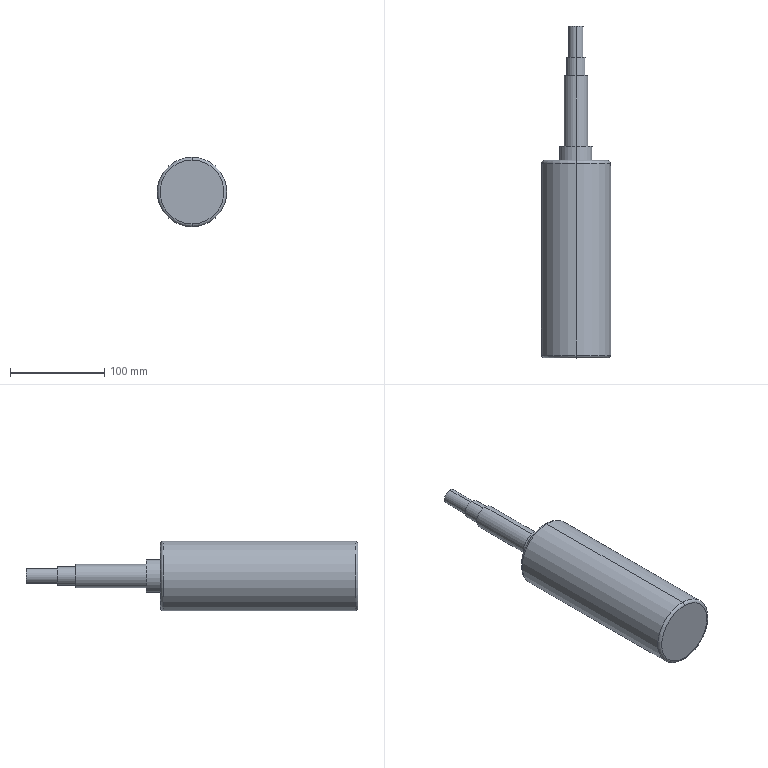Part | SolidWorks | features ICE 4, Extrusion 1, Fillet 1 | 1 solid | 20 faces | box 74 x 353 x 74 mm | volume 966460 mm3 | cylinder 10 | plane 6 | torus 4 | commonest cylinder face diameters 16 x2 20 x2 25 x2 35 x2 74 x2
STEP:
#1=CARTESIAN_POINT('',(0.,102.,-37.));
#2=VERTEX_POINT('',#1);
#3=CARTESIAN_POINT('',(0.,102.,37.));
#4=VERTEX_POINT('',#3);
#5=CARTESIAN_POINT('',(0.,102.,0.));
#6=DIRECTION('',(0.,-1.,0.));
#7=DIRECTION('',(0.,0.,1.));
#8=AXIS2_PLACEMENT_3D('',#5,#6,#7);
#9=CIRCLE('',#8,37.);
#10=EDGE_CURVE('',#2,#4,#9,.T.);
#11=ORIENTED_EDGE('',*,*,#10,.F.);
#12=CARTESIAN_POINT('',(0.,105.,-34.));
#13=VERTEX_POINT('',#12);
#14=CARTESIAN_POINT('',(0.,102.,-34.));
#15=DIRECTION('',(1.,0.,0.));
#16=DIRECTION('',(0.,0.,-1.));
#17=AXIS2_PLACEMENT_3D('',#14,#15,#16);
#18=CIRCLE('',#17,3.);
#19=EDGE_CURVE('',#2,#13,#18,.T.);
#20=ORIENTED_EDGE('',*,*,#19,.T.);
#21=CARTESIAN_POINT('',(0.,105.,34.));
#22=VERTEX_POINT('',#21);
#23=CARTESIAN_POINT('',(0.,105.,0.));
#24=DIRECTION('',(0.,1.,0.));
#25=DIRECTION('',(0.,0.,1.));
#26=AXIS2_PLACEMENT_3D('',#23,#24,#25);
#27=CIRCLE('',#26,34.);
#28=EDGE_CURVE('',#22,#13,#27,.T.);
#29=ORIENTED_EDGE('',*,*,#28,.F.);
#30=CARTESIAN_POINT('',(0.,102.,34.));
#31=DIRECTION('',(-1.,0.,0.));
#32=DIRECTION('',(0.,0.,1.));
#33=AXIS2_PLACEMENT_3D('',#30,#31,#32);
#34=CIRCLE('',#33,3.);
#35=EDGE_CURVE('',#4,#22,#34,.T.);
#36=ORIENTED_EDGE('',*,*,#35,.F.);
#37=EDGE_LOOP('',(#11,#20,#29,#36));
#38=FACE_OUTER_BOUND('',#37,.T.);
#39=CARTESIAN_POINT('',(0.,102.,0.));
#40=DIRECTION('',(0.,1.,0.));
#41=DIRECTION('',(0.,0.,1.));
#42=AXIS2_PLACEMENT_3D('',#39,#40,#41);
#43=TOROIDAL_SURFACE('',#42,34.,3.);
#44=ADVANCED_FACE('',(#38),#43,.T.);
#45=CARTESIAN_POINT('',(0.,-105.,-34.));
#46=VERTEX_POINT('',#45);
#47=CARTESIAN_POINT('',(0.,-105.,34.));
#48=VERTEX_POINT('',#47);
#49=CARTESIAN_POINT('',(0.,-105.,0.));
#50=DIRECTION('',(0.,-1.,0.));
#51=DIRECTION('',(0.,0.,1.));
#52=AXIS2_PLACEMENT_3D('',#49,#50,#51);
#53=CIRCLE('',#52,34.);
#54=EDGE_CURVE('',#46,#48,#53,.T.);
#55=ORIENTED_EDGE('',*,*,#54,.F.);
#56=CARTESIAN_POINT('',(0.,-102.,-37.));
#57=VERTEX_POINT('',#56);
#58=CARTESIAN_POINT('',(0.,-102.,-34.));
#59=DIRECTION('',(1.,0.,0.));
#60=DIRECTION('',(0.,0.,-1.));
#61=AXIS2_PLACEMENT_3D('',#58,#59,#60);
#62=CIRCLE('',#61,3.);
#63=EDGE_CURVE('',#46,#57,#62,.T.);
#64=ORIENTED_EDGE('',*,*,#63,.T.);
#65=CARTESIAN_POINT('',(0.,-102.,37.));
#66=VERTEX_POINT('',#65);
#67=CARTESIAN_POINT('',(0.,-102.,0.));
#68=DIRECTION('',(0.,1.,0.));
#69=DIRECTION('',(0.,0.,1.));
#70=AXIS2_PLACEMENT_3D('',#67,#68,#69);
#71=CIRCLE('',#70,37.);
#72=EDGE_CURVE('',#66,#57,#71,.T.);
#73=ORIENTED_EDGE('',*,*,#72,.F.);
#74=CARTESIAN_POINT('',(0.,-102.,34.));
#75=DIRECTION('',(-1.,0.,0.));
#76=DIRECTION('',(0.,0.,1.));
#77=AXIS2_PLACEMENT_3D('',#74,#75,#76);
#78=CIRCLE('',#77,3.);
#79=EDGE_CURVE('',#48,#66,#78,.T.);
#80=ORIENTED_EDGE('',*,*,#79,.F.);
#81=EDGE_LOOP('',(#55,#64,#73,#80));
#82=FACE_OUTER_BOUND('',#81,.T.);
#83=CARTESIAN_POINT('',(0.,-102.,0.));
#84=DIRECTION('',(0.,1.,0.));
#85=DIRECTION('',(0.,0.,1.));
#86=AXIS2_PLACEMENT_3D('',#83,#84,#85);
#87=TOROIDAL_SURFACE('',#86,34.,3.);
#88=ADVANCED_FACE('',(#82),#87,.T.);
#89=CARTESIAN_POINT('',(0.,248.,8.));
#90=VERTEX_POINT('',#89);
#91=CARTESIAN_POINT('',(0.,248.,-8.));
#92=VERTEX_POINT('',#91);
#93=CARTESIAN_POINT('',(0.,248.,0.));
#94=DIRECTION('',(0.,1.,0.));
#95=DIRECTION('',(0.,0.,1.));
#96=AXIS2_PLACEMENT_3D('',#93,#94,#95);
#97=CIRCLE('',#96,8.);
#98=EDGE_CURVE('',#90,#92,#97,.T.);
#99=ORIENTED_EDGE('',*,*,#98,.F.);
#100=CARTESIAN_POINT('',(0.,215.,8.));
#101=VERTEX_POINT('',#100);
#102=CARTESIAN_POINT('',(0.,248.,8.));
#103=DIRECTION('',(0.,-1.,0.));
#104=VECTOR('',#103,1000.);
#105=LINE('',#102,#104);
#106=EDGE_CURVE('',#90,#101,#105,.T.);
#107=ORIENTED_EDGE('',*,*,#106,.T.);
#108=CARTESIAN_POINT('',(0.,215.,-8.));
#109=VERTEX_POINT('',#108);
#110=CARTESIAN_POINT('',(0.,215.,0.));
#111=DIRECTION('',(0.,1.,0.));
#112=DIRECTION('',(0.,0.,1.));
#113=AXIS2_PLACEMENT_3D('',#110,#111,#112);
#114=CIRCLE('',#113,8.);
#115=EDGE_CURVE('',#101,#109,#114,.T.);
#116=ORIENTED_EDGE('',*,*,#115,.T.);
#117=CARTESIAN_POINT('',(0.,248.,-8.));
#118=DIRECTION('',(0.,-1.,0.));
#119=VECTOR('',#118,1000.);
#120=LINE('',#117,#119);
#121=EDGE_CURVE('',#92,#109,#120,.T.);
#122=ORIENTED_EDGE('',*,*,#121,.F.);
#123=EDGE_LOOP('',(#99,#107,#116,#122));
#124=FACE_OUTER_BOUND('',#123,.T.);
#125=CARTESIAN_POINT('',(0.,248.,0.));
#126=DIRECTION('',(0.,-1.,0.));
#127=DIRECTION('',(0.,0.,-1.));
#128=AXIS2_PLACEMENT_3D('',#125,#126,#127);
#129=CYLINDRICAL_SURFACE('',#128,8.);
#130=ADVANCED_FACE('',(#124),#129,.T.);
#131=CARTESIAN_POINT('',(0.,215.,10.));
#132=VERTEX_POINT('',#131);
#133=CARTESIAN_POINT('',(0.,215.,-10.));
#134=VERTEX_POINT('',#133);
#135=CARTESIAN_POINT('',(0.,215.,0.));
#136=DIRECTION('',(0.,1.,0.));
#137=DIRECTION('',(0.,0.,1.));
#138=AXIS2_PLACEMENT_3D('',#135,#136,#137);
#139=CIRCLE('',#138,10.);
#140=EDGE_CURVE('',#132,#134,#139,.T.);
#141=ORIENTED_EDGE('',*,*,#140,.F.);
#142=CARTESIAN_POINT('',(0.,195.,10.));
#143=VERTEX_POINT('',#142);
#144=CARTESIAN_POINT('',(0.,215.,10.));
#145=DIRECTION('',(0.,-1.,0.));
#146=VECTOR('',#145,1000.);
#147=LINE('',#144,#146);
#148=EDGE_CURVE('',#132,#143,#147,.T.);
#149=ORIENTED_EDGE('',*,*,#148,.T.);
#150=CARTESIAN_POINT('',(0.,195.,-10.));
#151=VERTEX_POINT('',#150);
#152=CARTESIAN_POINT('',(0.,195.,0.));
#153=DIRECTION('',(0.,1.,0.));
#154=DIRECTION('',(0.,0.,1.));
#155=AXIS2_PLACEMENT_3D('',#152,#153,#154);
#156=CIRCLE('',#155,10.);
#157=EDGE_CURVE('',#143,#151,#156,.T.);
#158=ORIENTED_EDGE('',*,*,#157,.T.);
#159=CARTESIAN_POINT('',(0.,215.,-10.));
#160=DIRECTION('',(0.,-1.,0.));
#161=VECTOR('',#160,1000.);
#162=LINE('',#159,#161);
#163=EDGE_CURVE('',#134,#151,#162,.T.);
#164=ORIENTED_EDGE('',*,*,#163,.F.);
#165=EDGE_LOOP('',(#141,#149,#158,#164));
#166=FACE_OUTER_BOUND('',#165,.T.);
#167=CARTESIAN_POINT('',(0.,215.,0.));
#168=DIRECTION('',(0.,-1.,0.));
#169=DIRECTION('',(0.,0.,-1.));
#170=AXIS2_PLACEMENT_3D('',#167,#168,#169);
#171=CYLINDRICAL_SURFACE('',#170,10.);
#172=ADVANCED_FACE('',(#166),#171,.T.);
#173=CARTESIAN_POINT('',(0.,195.,12.5));
#174=VERTEX_POINT('',#173);
#175=CARTESIAN_POINT('',(0.,195.,-12.5));
#176=VERTEX_POINT('',#175);
#177=CARTESIAN_POINT('',(0.,195.,0.));
#178=DIRECTION('',(0.,1.,0.));
#179=DIRECTION('',(0.,0.,1.));
#180=AXIS2_PLACEMENT_3D('',#177,#178,#179);
#181=CIRCLE('',#180,12.5);
#182=EDGE_CURVE('',#174,#176,#181,.T.);
#183=ORIENTED_EDGE('',*,*,#182,.F.);
#184=CARTESIAN_POINT('',(0.,120.,12.5));
#185=VERTEX_POINT('',#184);
#186=CARTESIAN_POINT('',(0.,195.,12.5));
#187=DIRECTION('',(0.,-1.,0.));
#188=VECTOR('',#187,1000.);
#189=LINE('',#186,#188);
#190=EDGE_CURVE('',#174,#185,#189,.T.);
#191=ORIENTED_EDGE('',*,*,#190,.T.);
#192=CARTESIAN_POINT('',(0.,120.,-12.5));
#193=VERTEX_POINT('',#192);
#194=CARTESIAN_POINT('',(0.,120.,0.));
#195=DIRECTION('',(0.,1.,0.));
#196=DIRECTION('',(0.,0.,1.));
#197=AXIS2_PLACEMENT_3D('',#194,#195,#196);
#198=CIRCLE('',#197,12.5);
#199=EDGE_CURVE('',#185,#193,#198,.T.);
#200=ORIENTED_EDGE('',*,*,#199,.T.);
#201=CARTESIAN_POINT('',(0.,195.,-12.5));
#202=DIRECTION('',(0.,-1.,0.));
#203=VECTOR('',#202,1000.);
#204=LINE('',#201,#203);
#205=EDGE_CURVE('',#176,#193,#204,.T.);
#206=ORIENTED_EDGE('',*,*,#205,.F.);
#207=EDGE_LOOP('',(#183,#191,#200,#206));
#208=FACE_OUTER_BOUND('',#207,.T.);
#209=CARTESIAN_POINT('',(0.,195.,0.));
#210=DIRECTION('',(0.,-1.,0.));
#211=DIRECTION('',(0.,0.,-1.));
#212=AXIS2_PLACEMENT_3D('',#209,#210,#211);
#213=CYLINDRICAL_SURFACE('',#212,12.5);
#214=ADVANCED_FACE('',(#208),#213,.T.);
#215=CARTESIAN_POINT('',(0.,120.,17.5));
#216=VERTEX_POINT('',#215);
#217=CARTESIAN_POINT('',(0.,120.,-17.5));
#218=VERTEX_POINT('',#217);
#219=CARTESIAN_POINT('',(0.,120.,0.));
#220=DIRECTION('',(0.,1.,0.));
#221=DIRECTION('',(0.,0.,1.));
#222=AXIS2_PLACEMENT_3D('',#219,#220,#221);
#223=CIRCLE('',#222,17.5);
#224=EDGE_CURVE('',#216,#218,#223,.T.);
#225=ORIENTED_EDGE('',*,*,#224,.F.);
#226=CARTESIAN_POINT('',(0.,105.,17.5));
#227=VERTEX_POINT('',#226);
#228=CARTESIAN_POINT('',(0.,120.,17.5));
#229=DIRECTION('',(0.,-1.,0.));
#230=VECTOR('',#229,1000.);
#231=LINE('',#228,#230);
#232=EDGE_CURVE('',#216,#227,#231,.T.);
#233=ORIENTED_EDGE('',*,*,#232,.T.);
#234=CARTESIAN_POINT('',(0.,105.,-17.5));
#235=VERTEX_POINT('',#234);
#236=CARTESIAN_POINT('',(0.,105.,0.));
#237=DIRECTION('',(0.,1.,0.));
#238=DIRECTION('',(0.,0.,1.));
#239=AXIS2_PLACEMENT_3D('',#236,#237,#238);
#240=CIRCLE('',#239,17.5);
#241=EDGE_CURVE('',#227,#235,#240,.T.);
#242=ORIENTED_EDGE('',*,*,#241,.T.);
#243=CARTESIAN_POINT('',(0.,120.,-17.5));
#244=DIRECTION('',(0.,-1.,0.));
#245=VECTOR('',#244,1000.);
#246=LINE('',#243,#245);
#247=EDGE_CURVE('',#218,#235,#246,.T.);
#248=ORIENTED_EDGE('',*,*,#247,.F.);
#249=EDGE_LOOP('',(#225,#233,#242,#248));
#250=FACE_OUTER_BOUND('',#249,.T.);
#251=CARTESIAN_POINT('',(0.,120.,0.));
#252=DIRECTION('',(0.,-1.,0.));
#253=DIRECTION('',(0.,0.,-1.));
#254=AXIS2_PLACEMENT_3D('',#251,#252,#253);
#255=CYLINDRICAL_SURFACE('',#254,17.5);
#256=ADVANCED_FACE('',(#250),#255,.T.);
#257=ORIENTED_EDGE('',*,*,#10,.T.);
#258=CARTESIAN_POINT('',(0.,105.,37.));
#259=DIRECTION('',(0.,-1.,0.));
#260=VECTOR('',#259,1000.);
#261=LINE('',#258,#260);
#262=EDGE_CURVE('',#4,#66,#261,.T.);
#263=ORIENTED_EDGE('',*,*,#262,.T.);
#264=ORIENTED_EDGE('',*,*,#72,.T.);
#265=CARTESIAN_POINT('',(0.,105.,-37.));
#266=DIRECTION('',(0.,-1.,0.));
#267=VECTOR('',#266,1000.);
#268=LINE('',#265,#267);
#269=EDGE_CURVE('',#2,#57,#268,.T.);
#270=ORIENTED_EDGE('',*,*,#269,.F.);
#271=EDGE_LOOP('',(#257,#263,#264,#270));
#272=FACE_OUTER_BOUND('',#271,.T.);
#273=CARTESIAN_POINT('',(0.,105.,0.));
#274=DIRECTION('',(0.,-1.,0.));
#275=DIRECTION('',(0.,0.,-1.));
#276=AXIS2_PLACEMENT_3D('',#273,#274,#275);
#277=CYLINDRICAL_SURFACE('',#276,37.);
#278=ADVANCED_FACE('',(#272),#277,.T.);
#279=ORIENTED_EDGE('',*,*,#262,.F.);
#280=CARTESIAN_POINT('',(0.,102.,0.));
#281=DIRECTION('',(0.,-1.,0.));
#282=DIRECTION('',(0.,0.,1.));
#283=AXIS2_PLACEMENT_3D('',#280,#281,#282);
#284=CIRCLE('',#283,37.);
#285=EDGE_CURVE('',#4,#2,#284,.T.);
#286=ORIENTED_EDGE('',*,*,#285,.T.);
#287=ORIENTED_EDGE('',*,*,#269,.T.);
#288=CARTESIAN_POINT('',(0.,-102.,0.));
#289=DIRECTION('',(0.,1.,0.));
#290=DIRECTION('',(0.,0.,1.));
#291=AXIS2_PLACEMENT_3D('',#288,#289,#290);
#292=CIRCLE('',#291,37.);
#293=EDGE_CURVE('',#57,#66,#292,.T.);
#294=ORIENTED_EDGE('',*,*,#293,.T.);
#295=EDGE_LOOP('',(#279,#286,#287,#294));
#296=FACE_OUTER_BOUND('',#295,.T.);
#297=CARTESIAN_POINT('',(0.,105.,0.));
#298=DIRECTION('',(0.,-1.,0.));
#299=DIRECTION('',(0.,0.,-1.));
#300=AXIS2_PLACEMENT_3D('',#297,#298,#299);
#301=CYLINDRICAL_SURFACE('',#300,37.);
#302=ADVANCED_FACE('',(#296),#301,.T.);
#303=ORIENTED_EDGE('',*,*,#28,.T.);
#304=CARTESIAN_POINT('',(0.,105.,0.));
#305=DIRECTION('',(0.,1.,0.));
#306=DIRECTION('',(0.,0.,1.));
#307=AXIS2_PLACEMENT_3D('',#304,#305,#306);
#308=CIRCLE('',#307,34.);
#309=EDGE_CURVE('',#13,#22,#308,.T.);
#310=ORIENTED_EDGE('',*,*,#309,.T.);
#311=EDGE_LOOP('',(#303,#310));
#312=FACE_OUTER_BOUND('',#311,.T.);
#313=CARTESIAN_POINT('',(0.,105.,0.));
#314=DIRECTION('',(0.,1.,0.));
#315=DIRECTION('',(0.,0.,1.));
#316=AXIS2_PLACEMENT_3D('',#313,#314,#315);
#317=CIRCLE('',#316,17.5);
#318=EDGE_CURVE('',#235,#227,#317,.T.);
#319=ORIENTED_EDGE('',*,*,#318,.F.);
#320=ORIENTED_EDGE('',*,*,#241,.F.);
#321=EDGE_LOOP('',(#319,#320));
#322=FACE_BOUND('',#321,.T.);
#323=CARTESIAN_POINT('',(0.,105.,0.));
#324=DIRECTION('',(0.,1.,0.));
#325=DIRECTION('',(0.,0.,1.));
#326=AXIS2_PLACEMENT_3D('',#323,#324,#325);
#327=PLANE('',#326);
#328=ADVANCED_FACE('',(#312,#322),#327,.T.);
#329=CARTESIAN_POINT('',(0.,-105.,0.));
#330=DIRECTION('',(0.,-1.,0.));
#331=DIRECTION('',(0.,0.,1.));
#332=AXIS2_PLACEMENT_3D('',#329,#330,#331);
#333=CIRCLE('',#332,34.);
#334=EDGE_CURVE('',#48,#46,#333,.T.);
#335=ORIENTED_EDGE('',*,*,#334,.T.);
#336=ORIENTED_EDGE('',*,*,#54,.T.);
#337=EDGE_LOOP('',(#335,#336));
#338=FACE_OUTER_BOUND('',#337,.T.);
#339=CARTESIAN_POINT('',(0.,-105.,0.));
#340=DIRECTION('',(0.,1.,0.));
#341=DIRECTION('',(0.,0.,1.));
#342=AXIS2_PLACEMENT_3D('',#339,#340,#341);
#343=PLANE('',#342);
#344=ADVANCED_FACE('',(#338),#343,.F.);
#345=ORIENTED_EDGE('',*,*,#232,.F.);
#346=CARTESIAN_POINT('',(0.,120.,0.));
#347=DIRECTION('',(0.,1.,0.));
#348=DIRECTION('',(0.,0.,1.));
#349=AXIS2_PLACEMENT_3D('',#346,#347,#348);
#350=CIRCLE('',#349,17.5);
#351=EDGE_CURVE('',#218,#216,#350,.T.);
#352=ORIENTED_EDGE('',*,*,#351,.F.);
#353=ORIENTED_EDGE('',*,*,#247,.T.);
#354=ORIENTED_EDGE('',*,*,#318,.T.);
#355=EDGE_LOOP('',(#345,#352,#353,#354));
#356=FACE_OUTER_BOUND('',#355,.T.);
#357=CARTESIAN_POINT('',(0.,120.,0.));
#358=DIRECTION('',(0.,-1.,0.));
#359=DIRECTION('',(0.,0.,-1.));
#360=AXIS2_PLACEMENT_3D('',#357,#358,#359);
#361=CYLINDRICAL_SURFACE('',#360,17.5);
#362=ADVANCED_FACE('',(#356),#361,.T.);
#363=CARTESIAN_POINT('',(0.,120.,0.));
#364=DIRECTION('',(0.,1.,0.));
#365=DIRECTION('',(0.,0.,1.));
#366=AXIS2_PLACEMENT_3D('',#363,#364,#365);
#367=CIRCLE('',#366,12.5);
#368=EDGE_CURVE('',#193,#185,#367,.T.);
#369=ORIENTED_EDGE('',*,*,#368,.F.);
#370=ORIENTED_EDGE('',*,*,#199,.F.);
#371=EDGE_LOOP('',(#369,#370));
#372=FACE_BOUND('',#371,.T.);
#373=ORIENTED_EDGE('',*,*,#351,.T.);
#374=ORIENTED_EDGE('',*,*,#224,.T.);
#375=EDGE_LOOP('',(#373,#374));
#376=FACE_OUTER_BOUND('',#375,.T.);
#377=CARTESIAN_POINT('',(0.,120.,0.));
#378=DIRECTION('',(0.,1.,0.));
#379=DIRECTION('',(0.,0.,1.));
#380=AXIS2_PLACEMENT_3D('',#377,#378,#379);
#381=PLANE('',#380);
#382=ADVANCED_FACE('',(#372,#376),#381,.T.);
#383=ORIENTED_EDGE('',*,*,#190,.F.);
#384=CARTESIAN_POINT('',(0.,195.,0.));
#385=DIRECTION('',(0.,1.,0.));
#386=DIRECTION('',(0.,0.,1.));
#387=AXIS2_PLACEMENT_3D('',#384,#385,#386);
#388=CIRCLE('',#387,12.5);
#389=EDGE_CURVE('',#176,#174,#388,.T.);
#390=ORIENTED_EDGE('',*,*,#389,.F.);
#391=ORIENTED_EDGE('',*,*,#205,.T.);
#392=ORIENTED_EDGE('',*,*,#368,.T.);
#393=EDGE_LOOP('',(#383,#390,#391,#392));
#394=FACE_OUTER_BOUND('',#393,.T.);
#395=CARTESIAN_POINT('',(0.,195.,0.));
#396=DIRECTION('',(0.,-1.,0.));
#397=DIRECTION('',(0.,0.,-1.));
#398=AXIS2_PLACEMENT_3D('',#395,#396,#397);
#399=CYLINDRICAL_SURFACE('',#398,12.5);
#400=ADVANCED_FACE('',(#394),#399,.T.);
#401=CARTESIAN_POINT('',(0.,195.,0.));
#402=DIRECTION('',(0.,1.,0.));
#403=DIRECTION('',(0.,0.,1.));
#404=AXIS2_PLACEMENT_3D('',#401,#402,#403);
#405=CIRCLE('',#404,10.);
#406=EDGE_CURVE('',#151,#143,#405,.T.);
#407=ORIENTED_EDGE('',*,*,#406,.F.);
#408=ORIENTED_EDGE('',*,*,#157,.F.);
#409=EDGE_LOOP('',(#407,#408));
#410=FACE_BOUND('',#409,.T.);
#411=ORIENTED_EDGE('',*,*,#389,.T.);
#412=ORIENTED_EDGE('',*,*,#182,.T.);
#413=EDGE_LOOP('',(#411,#412));
#414=FACE_OUTER_BOUND('',#413,.T.);
#415=CARTESIAN_POINT('',(0.,195.,0.));
#416=DIRECTION('',(0.,1.,0.));
#417=DIRECTION('',(0.,0.,1.));
#418=AXIS2_PLACEMENT_3D('',#415,#416,#417);
#419=PLANE('',#418);
#420=ADVANCED_FACE('',(#410,#414),#419,.T.);
#421=ORIENTED_EDGE('',*,*,#148,.F.);
#422=CARTESIAN_POINT('',(0.,215.,0.));
#423=DIRECTION('',(0.,1.,0.));
#424=DIRECTION('',(0.,0.,1.));
#425=AXIS2_PLACEMENT_3D('',#422,#423,#424);
#426=CIRCLE('',#425,10.);
#427=EDGE_CURVE('',#134,#132,#426,.T.);
#428=ORIENTED_EDGE('',*,*,#427,.F.);
#429=ORIENTED_EDGE('',*,*,#163,.T.);
#430=ORIENTED_EDGE('',*,*,#406,.T.);
#431=EDGE_LOOP('',(#421,#428,#429,#430));
#432=FACE_OUTER_BOUND('',#431,.T.);
#433=CARTESIAN_POINT('',(0.,215.,0.));
#434=DIRECTION('',(0.,-1.,0.));
#435=DIRECTION('',(0.,0.,-1.));
#436=AXIS2_PLACEMENT_3D('',#433,#434,#435);
#437=CYLINDRICAL_SURFACE('',#436,10.);
#438=ADVANCED_FACE('',(#432),#437,.T.);
#439=CARTESIAN_POINT('',(0.,215.,0.));
#440=DIRECTION('',(0.,1.,0.));
#441=DIRECTION('',(0.,0.,1.));
#442=AXIS2_PLACEMENT_3D('',#439,#440,#441);
#443=CIRCLE('',#442,8.);
#444=EDGE_CURVE('',#109,#101,#443,.T.);
#445=ORIENTED_EDGE('',*,*,#444,.F.);
#446=ORIENTED_EDGE('',*,*,#115,.F.);
#447=EDGE_LOOP('',(#445,#446));
#448=FACE_BOUND('',#447,.T.);
#449=ORIENTED_EDGE('',*,*,#427,.T.);
#450=ORIENTED_EDGE('',*,*,#140,.T.);
#451=EDGE_LOOP('',(#449,#450));
#452=FACE_OUTER_BOUND('',#451,.T.);
#453=CARTESIAN_POINT('',(0.,215.,0.));
#454=DIRECTION('',(0.,1.,0.));
#455=DIRECTION('',(0.,0.,1.));
#456=AXIS2_PLACEMENT_3D('',#453,#454,#455);
#457=PLANE('',#456);
#458=ADVANCED_FACE('',(#448,#452),#457,.T.);
#459=ORIENTED_EDGE('',*,*,#106,.F.);
#460=CARTESIAN_POINT('',(0.,248.,0.));
#461=DIRECTION('',(0.,1.,0.));
#462=DIRECTION('',(0.,0.,1.));
#463=AXIS2_PLACEMENT_3D('',#460,#461,#462);
#464=CIRCLE('',#463,8.);
#465=EDGE_CURVE('',#92,#90,#464,.T.);
#466=ORIENTED_EDGE('',*,*,#465,.F.);
#467=ORIENTED_EDGE('',*,*,#121,.T.);
#468=ORIENTED_EDGE('',*,*,#444,.T.);
#469=EDGE_LOOP('',(#459,#466,#467,#468));
#470=FACE_OUTER_BOUND('',#469,.T.);
#471=CARTESIAN_POINT('',(0.,248.,0.));
#472=DIRECTION('',(0.,-1.,0.));
#473=DIRECTION('',(0.,0.,-1.));
#474=AXIS2_PLACEMENT_3D('',#471,#472,#473);
#475=CYLINDRICAL_SURFACE('',#474,8.);
#476=ADVANCED_FACE('',(#470),#475,.T.);
#477=ORIENTED_EDGE('',*,*,#465,.T.);
#478=ORIENTED_EDGE('',*,*,#98,.T.);
#479=EDGE_LOOP('',(#477,#478));
#480=FACE_OUTER_BOUND('',#479,.T.);
#481=CARTESIAN_POINT('',(0.,248.,0.));
#482=DIRECTION('',(0.,1.,0.));
#483=DIRECTION('',(0.,0.,1.));
#484=AXIS2_PLACEMENT_3D('',#481,#482,#483);
#485=PLANE('',#484);
#486=ADVANCED_FACE('',(#480),#485,.T.);
#487=ORIENTED_EDGE('',*,*,#63,.F.);
#488=ORIENTED_EDGE('',*,*,#334,.F.);
#489=ORIENTED_EDGE('',*,*,#79,.T.);
#490=ORIENTED_EDGE('',*,*,#293,.F.);
#491=EDGE_LOOP('',(#487,#488,#489,#490));
#492=FACE_OUTER_BOUND('',#491,.T.);
#493=CARTESIAN_POINT('',(0.,-102.,0.));
#494=DIRECTION('',(0.,1.,0.));
#495=DIRECTION('',(0.,0.,1.));
#496=AXIS2_PLACEMENT_3D('',#493,#494,#495);
#497=TOROIDAL_SURFACE('',#496,34.,3.);
#498=ADVANCED_FACE('',(#492),#497,.T.);
#499=ORIENTED_EDGE('',*,*,#19,.F.);
#500=ORIENTED_EDGE('',*,*,#285,.F.);
#501=ORIENTED_EDGE('',*,*,#35,.T.);
#502=ORIENTED_EDGE('',*,*,#309,.F.);
#503=EDGE_LOOP('',(#499,#500,#501,#502));
#504=FACE_OUTER_BOUND('',#503,.T.);
#505=CARTESIAN_POINT('',(0.,102.,0.));
#506=DIRECTION('',(0.,1.,0.));
#507=DIRECTION('',(0.,0.,1.));
#508=AXIS2_PLACEMENT_3D('',#505,#506,#507);
#509=TOROIDAL_SURFACE('',#508,34.,3.);
#510=ADVANCED_FACE('',(#504),#509,.T.);
#511=CLOSED_SHELL('',(#44,#88,#130,#172,#214,#256,#278,#302,#328,#344,#362,#382,#400,#420,#438,#458,#476,#486,#498,#510));
#512=MANIFOLD_SOLID_BREP('',#511);
#513=CARTESIAN_POINT('',(0.,0.,0.));
#514=DIRECTION('',(0.,0.,1.));
#515=DIRECTION('',(1.,0.,0.));
#516=AXIS2_PLACEMENT_3D('',#513,#514,#515);
#517=(LENGTH_UNIT()NAMED_UNIT(*)SI_UNIT(.MILLI.,.METRE.));
#518=UNCERTAINTY_MEASURE_WITH_UNIT(LENGTH_MEASURE(0.00001),#517,'','');
#519=(NAMED_UNIT(*)PLANE_ANGLE_UNIT()SI_UNIT($,.RADIAN.));
#520=(NAMED_UNIT(*)SI_UNIT($,.STERADIAN.)SOLID_ANGLE_UNIT());
#521=(GEOMETRIC_REPRESENTATION_CONTEXT(3)GLOBAL_UNCERTAINTY_ASSIGNED_CONTEXT((#518))GLOBAL_UNIT_ASSIGNED_CONTEXT((#517,#519,#520))REPRESENTATION_CONTEXT('',''));
#522=ADVANCED_BREP_SHAPE_REPRESENTATION('',(#512,#516),#521);